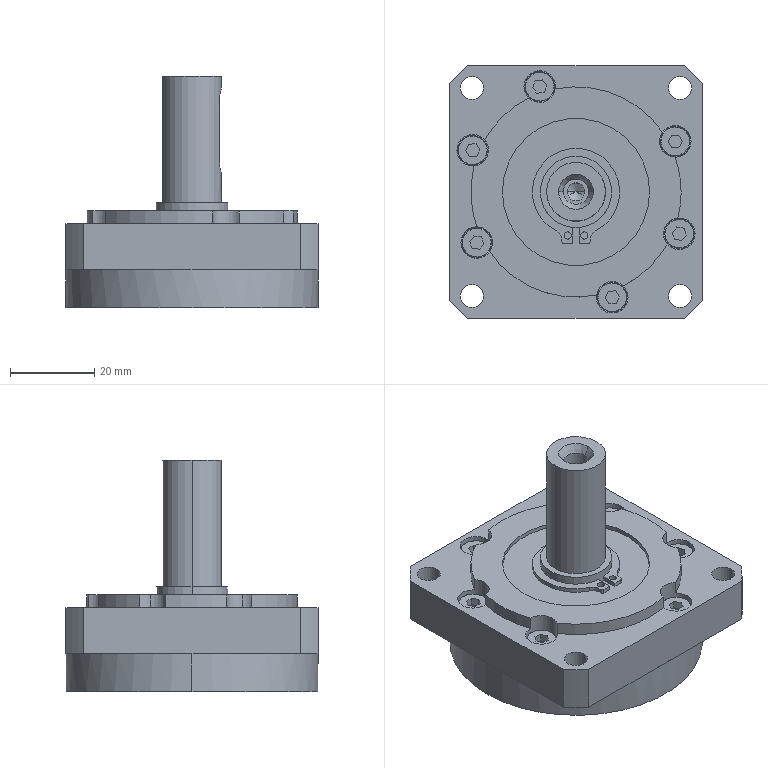Part | STEP file | 1 solid | 169 faces | box 60 x 60 x 55 mm | volume 72003 mm3 | plane 82 | cylinder 71 | spline 12 | cone 4 | commonest cylinder face diameters 7 x12 7.5 x12 5.5 x8 50 x7 5 x5 1.7 x4